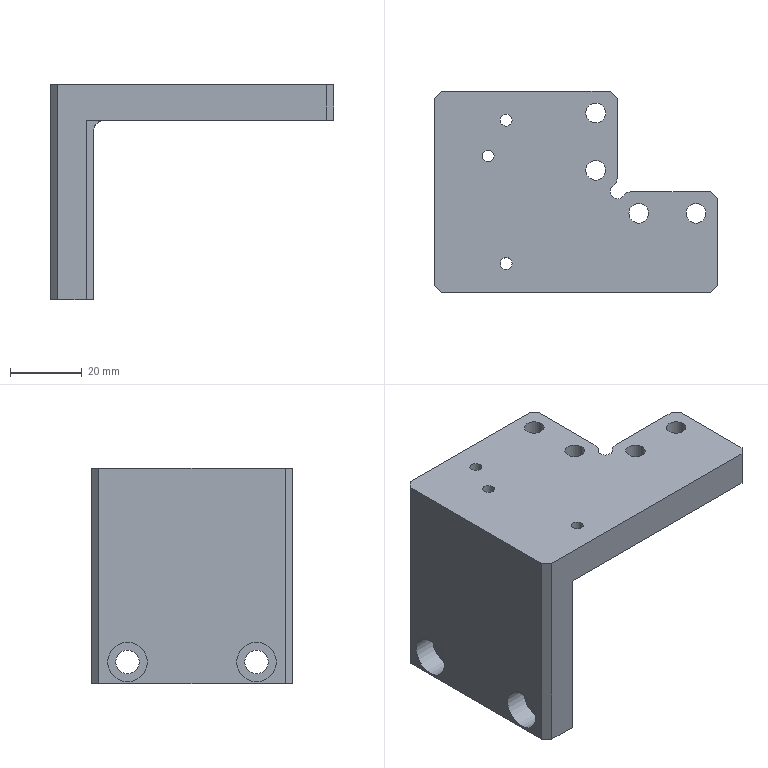Part | 1 solid | 42 faces | box 79 x 56 x 60 mm | volume 65502 mm3 | plane 23 | cylinder 19 | commonest cylinder face diameters 5.5 x4 10 x4 3.3 x3 6 x3 6.6 x2 11 x2
STEP:
#1=CARTESIAN_POINT('',(10.3,1.6,20.));
#2=VERTEX_POINT('',#1);
#3=CARTESIAN_POINT('',(13.1,-1.2,20.));
#4=VERTEX_POINT('',#3);
#5=CARTESIAN_POINT('',(11.5,0.,20.));
#6=DIRECTION('',(0.,0.,1.));
#7=DIRECTION('',(1.,0.,0.));
#8=AXIS2_PLACEMENT_3D('',#5,#6,#7);
#9=CIRCLE('',#8,2.);
#10=EDGE_CURVE('',#2,#4,#9,.T.);
#11=ORIENTED_EDGE('',*,*,#10,.F.);
#12=CARTESIAN_POINT('',(10.3,1.6,30.));
#13=VERTEX_POINT('',#12);
#14=CARTESIAN_POINT('',(10.3,1.6,20.));
#15=DIRECTION('',(0.,0.,1.));
#16=VECTOR('',#15,1000.);
#17=LINE('',#14,#16);
#18=EDGE_CURVE('',#2,#13,#17,.T.);
#19=ORIENTED_EDGE('',*,*,#18,.T.);
#20=CARTESIAN_POINT('',(13.1,-1.2,30.));
#21=VERTEX_POINT('',#20);
#22=CARTESIAN_POINT('',(11.5,0.,30.));
#23=DIRECTION('',(0.,0.,1.));
#24=DIRECTION('',(1.,0.,0.));
#25=AXIS2_PLACEMENT_3D('',#22,#23,#24);
#26=CIRCLE('',#25,2.);
#27=EDGE_CURVE('',#13,#21,#26,.T.);
#28=ORIENTED_EDGE('',*,*,#27,.T.);
#29=CARTESIAN_POINT('',(13.1,-1.2,20.));
#30=DIRECTION('',(0.,0.,1.));
#31=VECTOR('',#30,1000.);
#32=LINE('',#29,#31);
#33=EDGE_CURVE('',#21,#4,#32,.F.);
#34=ORIENTED_EDGE('',*,*,#33,.T.);
#35=EDGE_LOOP('',(#11,#19,#28,#34));
#36=FACE_BOUND('',#35,.T.);
#37=CARTESIAN_POINT('',(11.5,0.,20.));
#38=DIRECTION('',(0.,0.,1.));
#39=DIRECTION('',(1.,0.,0.));
#40=AXIS2_PLACEMENT_3D('',#37,#38,#39);
#41=CYLINDRICAL_SURFACE('',#40,2.);
#42=ADVANCED_FACE('',(#36),#41,.F.);
#43=CARTESIAN_POINT('',(-33.1,18.,-29.5));
#44=VERTEX_POINT('',#43);
#45=CARTESIAN_POINT('',(-33.1,18.,-24.));
#46=DIRECTION('',(-1.,0.,0.));
#47=DIRECTION('',(0.,0.,-1.));
#48=AXIS2_PLACEMENT_3D('',#45,#46,#47);
#49=CIRCLE('',#48,5.5);
#50=EDGE_CURVE('',#44,#44,#49,.T.);
#51=ORIENTED_EDGE('',*,*,#50,.T.);
#52=EDGE_LOOP('',(#51));
#53=FACE_BOUND('',#52,.T.);
#54=CARTESIAN_POINT('',(-33.1,18.,-27.3));
#55=VERTEX_POINT('',#54);
#56=CARTESIAN_POINT('',(-33.1,18.,-24.));
#57=DIRECTION('',(-1.,0.,0.));
#58=DIRECTION('',(0.,0.,-1.));
#59=AXIS2_PLACEMENT_3D('',#56,#57,#58);
#60=CIRCLE('',#59,3.3);
#61=EDGE_CURVE('',#55,#55,#60,.T.);
#62=ORIENTED_EDGE('',*,*,#61,.F.);
#63=EDGE_LOOP('',(#62));
#64=FACE_BOUND('',#63,.T.);
#65=CARTESIAN_POINT('',(-33.1,-14.7,-24.));
#66=DIRECTION('',(1.,0.,0.));
#67=DIRECTION('',(0.,0.,-1.));
#68=AXIS2_PLACEMENT_3D('',#65,#66,#67);
#69=PLANE('',#68);
#70=ADVANCED_FACE('',(#53,#64),#69,.F.);
#71=CARTESIAN_POINT('',(-33.1,-18.,-18.5));
#72=VERTEX_POINT('',#71);
#73=CARTESIAN_POINT('',(-33.1,-18.,-24.));
#74=DIRECTION('',(-1.,0.,0.));
#75=DIRECTION('',(0.,0.,1.));
#76=AXIS2_PLACEMENT_3D('',#73,#74,#75);
#77=CIRCLE('',#76,5.5);
#78=EDGE_CURVE('',#72,#72,#77,.T.);
#79=ORIENTED_EDGE('',*,*,#78,.T.);
#80=EDGE_LOOP('',(#79));
#81=FACE_BOUND('',#80,.T.);
#82=CARTESIAN_POINT('',(-33.1,-18.,-20.7));
#83=VERTEX_POINT('',#82);
#84=CARTESIAN_POINT('',(-33.1,-18.,-24.));
#85=DIRECTION('',(-1.,0.,0.));
#86=DIRECTION('',(0.,0.,1.));
#87=AXIS2_PLACEMENT_3D('',#84,#85,#86);
#88=CIRCLE('',#87,3.3);
#89=EDGE_CURVE('',#83,#83,#88,.T.);
#90=ORIENTED_EDGE('',*,*,#89,.F.);
#91=EDGE_LOOP('',(#90));
#92=FACE_BOUND('',#91,.T.);
#93=CARTESIAN_POINT('',(-33.1,-14.7,-24.));
#94=DIRECTION('',(1.,0.,0.));
#95=DIRECTION('',(0.,0.,-1.));
#96=AXIS2_PLACEMENT_3D('',#93,#94,#95);
#97=PLANE('',#96);
#98=ADVANCED_FACE('',(#81,#92),#97,.F.);
#99=CARTESIAN_POINT('',(-24.5,11.65,20.));
#100=VERTEX_POINT('',#99);
#101=CARTESIAN_POINT('',(-24.5,23.,20.));
#102=VERTEX_POINT('',#101);
#103=CARTESIAN_POINT('',(-24.5,26.,20.));
#104=DIRECTION('',(0.,1.,0.));
#105=VECTOR('',#104,1000.);
#106=LINE('',#103,#105);
#107=EDGE_CURVE('',#100,#102,#106,.T.);
#108=ORIENTED_EDGE('',*,*,#107,.F.);
#109=CARTESIAN_POINT('',(-24.5,8.35,20.));
#110=VERTEX_POINT('',#109);
#111=CARTESIAN_POINT('',(-24.5,11.65,20.));
#112=CARTESIAN_POINT('',(-24.946,11.65,20.));
#113=CARTESIAN_POINT('',(-25.788,11.29,19.774));
#114=CARTESIAN_POINT('',(-26.331,10.001,19.371));
#115=CARTESIAN_POINT('',(-25.788,8.709,19.774));
#116=CARTESIAN_POINT('',(-24.946,8.35,20.));
#117=CARTESIAN_POINT('',(-24.5,8.35,20.));
#118=B_SPLINE_CURVE_WITH_KNOTS('',3,(#111,#112,#113,#114,#115,#116,#117),.UNSPECIFIED.,.F.,.F.,(4,1,1,1,4),(-0.002635,-0.001318,-0.000000456,0.001317,0.002634),.UNSPECIFIED.);
#119=EDGE_CURVE('',#100,#110,#118,.T.);
#120=ORIENTED_EDGE('',*,*,#119,.T.);
#121=CARTESIAN_POINT('',(-24.5,-23.,20.));
#122=VERTEX_POINT('',#121);
#123=CARTESIAN_POINT('',(-24.5,26.,20.));
#124=DIRECTION('',(0.,1.,0.));
#125=VECTOR('',#124,1000.);
#126=LINE('',#123,#125);
#127=EDGE_CURVE('',#122,#110,#126,.T.);
#128=ORIENTED_EDGE('',*,*,#127,.F.);
#129=CARTESIAN_POINT('',(-27.5,-26.,17.));
#130=VERTEX_POINT('',#129);
#131=CARTESIAN_POINT('',(-24.5,-23.,17.));
#132=DIRECTION('',(-0.7071,0.7071,0.));
#133=DIRECTION('',(0.7071,0.7071,0.));
#134=AXIS2_PLACEMENT_3D('',#131,#132,#133);
#135=ELLIPSE('',#134,4.243,3.);
#136=EDGE_CURVE('',#130,#122,#135,.T.);
#137=ORIENTED_EDGE('',*,*,#136,.F.);
#138=CARTESIAN_POINT('',(-27.5,26.,17.));
#139=VERTEX_POINT('',#138);
#140=CARTESIAN_POINT('',(-27.5,-26.,17.));
#141=DIRECTION('',(0.,-1.,0.));
#142=VECTOR('',#141,1000.);
#143=LINE('',#140,#142);
#144=EDGE_CURVE('',#139,#130,#143,.T.);
#145=ORIENTED_EDGE('',*,*,#144,.F.);
#146=CARTESIAN_POINT('',(-24.5,23.,17.));
#147=DIRECTION('',(-0.7071,-0.7071,0.));
#148=DIRECTION('',(-0.7071,0.7071,0.));
#149=AXIS2_PLACEMENT_3D('',#146,#147,#148);
#150=ELLIPSE('',#149,4.243,3.);
#151=EDGE_CURVE('',#102,#139,#150,.T.);
#152=ORIENTED_EDGE('',*,*,#151,.F.);
#153=EDGE_LOOP('',(#108,#120,#128,#137,#145,#152));
#154=FACE_BOUND('',#153,.T.);
#155=CARTESIAN_POINT('',(-24.5,28.,17.));
#156=DIRECTION('',(0.,1.,0.));
#157=DIRECTION('',(0.,0.,1.));
#158=AXIS2_PLACEMENT_3D('',#155,#156,#157);
#159=CYLINDRICAL_SURFACE('',#158,3.);
#160=ADVANCED_FACE('',(#154),#159,.F.);
#161=CARTESIAN_POINT('',(-37.5,28.,30.));
#162=VERTEX_POINT('',#161);
#163=CARTESIAN_POINT('',(-39.5,26.,30.));
#164=VERTEX_POINT('',#163);
#165=CARTESIAN_POINT('',(-32.75,32.75,30.));
#166=DIRECTION('',(-0.7071,-0.7071,0.));
#167=VECTOR('',#166,1000.);
#168=LINE('',#165,#167);
#169=EDGE_CURVE('',#162,#164,#168,.T.);
#170=ORIENTED_EDGE('',*,*,#169,.F.);
#171=CARTESIAN_POINT('',(-37.5,28.,-30.));
#172=VERTEX_POINT('',#171);
#173=CARTESIAN_POINT('',(-37.5,28.,30.));
#174=DIRECTION('',(0.,0.,1.));
#175=VECTOR('',#174,1000.);
#176=LINE('',#173,#175);
#177=EDGE_CURVE('',#172,#162,#176,.T.);
#178=ORIENTED_EDGE('',*,*,#177,.F.);
#179=CARTESIAN_POINT('',(-39.5,26.,-30.));
#180=VERTEX_POINT('',#179);
#181=CARTESIAN_POINT('',(-39.5,26.,-30.));
#182=DIRECTION('',(0.7071,0.7071,0.));
#183=VECTOR('',#182,1000.);
#184=LINE('',#181,#183);
#185=EDGE_CURVE('',#180,#172,#184,.T.);
#186=ORIENTED_EDGE('',*,*,#185,.F.);
#187=CARTESIAN_POINT('',(-39.5,26.,30.));
#188=DIRECTION('',(0.,0.,-1.));
#189=VECTOR('',#188,1000.);
#190=LINE('',#187,#189);
#191=EDGE_CURVE('',#164,#180,#190,.T.);
#192=ORIENTED_EDGE('',*,*,#191,.F.);
#193=EDGE_LOOP('',(#170,#178,#186,#192));
#194=FACE_BOUND('',#193,.T.);
#195=CARTESIAN_POINT('',(-39.5,26.,30.));
#196=DIRECTION('',(0.7071,-0.7071,0.));
#197=DIRECTION('',(0.,0.,-1.));
#198=AXIS2_PLACEMENT_3D('',#195,#196,#197);
#199=PLANE('',#198);
#200=ADVANCED_FACE('',(#194),#199,.F.);
#201=CARTESIAN_POINT('',(-29.5,28.,20.));
#202=VERTEX_POINT('',#201);
#203=CARTESIAN_POINT('',(5.,-6.5,20.));
#204=DIRECTION('',(-0.7071,0.7071,0.));
#205=VECTOR('',#204,1000.);
#206=LINE('',#203,#205);
#207=EDGE_CURVE('',#102,#202,#206,.T.);
#208=ORIENTED_EDGE('',*,*,#207,.F.);
#209=ORIENTED_EDGE('',*,*,#151,.T.);
#210=CARTESIAN_POINT('',(-27.5,26.,-30.));
#211=VERTEX_POINT('',#210);
#212=CARTESIAN_POINT('',(-27.5,26.,-30.));
#213=DIRECTION('',(0.,0.,1.));
#214=VECTOR('',#213,1000.);
#215=LINE('',#212,#214);
#216=EDGE_CURVE('',#211,#139,#215,.T.);
#217=ORIENTED_EDGE('',*,*,#216,.F.);
#218=CARTESIAN_POINT('',(-29.5,28.,-30.));
#219=VERTEX_POINT('',#218);
#220=CARTESIAN_POINT('',(-29.5,28.,-30.));
#221=DIRECTION('',(0.7071,-0.7071,0.));
#222=VECTOR('',#221,1000.);
#223=LINE('',#220,#222);
#224=EDGE_CURVE('',#219,#211,#223,.T.);
#225=ORIENTED_EDGE('',*,*,#224,.F.);
#226=CARTESIAN_POINT('',(-29.5,28.,30.));
#227=DIRECTION('',(0.,0.,-1.));
#228=VECTOR('',#227,1000.);
#229=LINE('',#226,#228);
#230=EDGE_CURVE('',#202,#219,#229,.T.);
#231=ORIENTED_EDGE('',*,*,#230,.F.);
#232=EDGE_LOOP('',(#208,#209,#217,#225,#231));
#233=FACE_BOUND('',#232,.T.);
#234=CARTESIAN_POINT('',(-29.5,28.,30.));
#235=DIRECTION('',(-0.7071,-0.7071,0.));
#236=DIRECTION('',(0.,0.,-1.));
#237=AXIS2_PLACEMENT_3D('',#234,#235,#236);
#238=PLANE('',#237);
#239=ADVANCED_FACE('',(#233),#238,.F.);
#240=CARTESIAN_POINT('',(-39.5,-26.,30.));
#241=VERTEX_POINT('',#240);
#242=CARTESIAN_POINT('',(-37.5,-28.,30.));
#243=VERTEX_POINT('',#242);
#244=CARTESIAN_POINT('',(-32.75,-32.75,30.));
#245=DIRECTION('',(0.7071,-0.7071,0.));
#246=VECTOR('',#245,1000.);
#247=LINE('',#244,#246);
#248=EDGE_CURVE('',#241,#243,#247,.T.);
#249=ORIENTED_EDGE('',*,*,#248,.F.);
#250=CARTESIAN_POINT('',(-39.5,-26.,-30.));
#251=VERTEX_POINT('',#250);
#252=CARTESIAN_POINT('',(-39.5,-26.,30.));
#253=DIRECTION('',(0.,0.,1.));
#254=VECTOR('',#253,1000.);
#255=LINE('',#252,#254);
#256=EDGE_CURVE('',#251,#241,#255,.T.);
#257=ORIENTED_EDGE('',*,*,#256,.F.);
#258=CARTESIAN_POINT('',(-37.5,-28.,-30.));
#259=VERTEX_POINT('',#258);
#260=CARTESIAN_POINT('',(-37.5,-28.,-30.));
#261=DIRECTION('',(-0.7071,0.7071,0.));
#262=VECTOR('',#261,1000.);
#263=LINE('',#260,#262);
#264=EDGE_CURVE('',#259,#251,#263,.T.);
#265=ORIENTED_EDGE('',*,*,#264,.F.);
#266=CARTESIAN_POINT('',(-37.5,-28.,30.));
#267=DIRECTION('',(0.,0.,-1.));
#268=VECTOR('',#267,1000.);
#269=LINE('',#266,#268);
#270=EDGE_CURVE('',#243,#259,#269,.T.);
#271=ORIENTED_EDGE('',*,*,#270,.F.);
#272=EDGE_LOOP('',(#249,#257,#265,#271));
#273=FACE_BOUND('',#272,.T.);
#274=CARTESIAN_POINT('',(-37.5,-28.,30.));
#275=DIRECTION('',(0.7071,0.7071,0.));
#276=DIRECTION('',(0.,0.,-1.));
#277=AXIS2_PLACEMENT_3D('',#274,#275,#276);
#278=PLANE('',#277);
#279=ADVANCED_FACE('',(#273),#278,.F.);
#280=CARTESIAN_POINT('',(-29.5,-28.,20.));
#281=VERTEX_POINT('',#280);
#282=CARTESIAN_POINT('',(33.,34.5,20.));
#283=DIRECTION('',(0.7071,0.7071,0.));
#284=VECTOR('',#283,1000.);
#285=LINE('',#282,#284);
#286=EDGE_CURVE('',#281,#122,#285,.T.);
#287=ORIENTED_EDGE('',*,*,#286,.F.);
#288=CARTESIAN_POINT('',(-29.5,-28.,-30.));
#289=VERTEX_POINT('',#288);
#290=CARTESIAN_POINT('',(-29.5,-28.,30.));
#291=DIRECTION('',(0.,0.,1.));
#292=VECTOR('',#291,1000.);
#293=LINE('',#290,#292);
#294=EDGE_CURVE('',#289,#281,#293,.T.);
#295=ORIENTED_EDGE('',*,*,#294,.F.);
#296=CARTESIAN_POINT('',(-27.5,-26.,-30.));
#297=VERTEX_POINT('',#296);
#298=CARTESIAN_POINT('',(-27.5,-26.,-30.));
#299=DIRECTION('',(-0.7071,-0.7071,0.));
#300=VECTOR('',#299,1000.);
#301=LINE('',#298,#300);
#302=EDGE_CURVE('',#297,#289,#301,.T.);
#303=ORIENTED_EDGE('',*,*,#302,.F.);
#304=CARTESIAN_POINT('',(-27.5,-26.,-30.));
#305=DIRECTION('',(0.,0.,-1.));
#306=VECTOR('',#305,1000.);
#307=LINE('',#304,#306);
#308=EDGE_CURVE('',#130,#297,#307,.T.);
#309=ORIENTED_EDGE('',*,*,#308,.F.);
#310=ORIENTED_EDGE('',*,*,#136,.T.);
#311=EDGE_LOOP('',(#287,#295,#303,#309,#310));
#312=FACE_BOUND('',#311,.T.);
#313=CARTESIAN_POINT('',(-27.5,-26.,-30.));
#314=DIRECTION('',(-0.7071,0.7071,0.));
#315=DIRECTION('',(0.,0.,-1.));
#316=AXIS2_PLACEMENT_3D('',#313,#314,#315);
#317=PLANE('',#316);
#318=ADVANCED_FACE('',(#312),#317,.F.);
#319=CARTESIAN_POINT('',(37.5,-28.,30.));
#320=VERTEX_POINT('',#319);
#321=CARTESIAN_POINT('',(39.5,-26.,30.));
#322=VERTEX_POINT('',#321);
#323=CARTESIAN_POINT('',(32.75,-32.75,30.));
#324=DIRECTION('',(0.7071,0.7071,0.));
#325=VECTOR('',#324,1000.);
#326=LINE('',#323,#325);
#327=EDGE_CURVE('',#320,#322,#326,.T.);
#328=ORIENTED_EDGE('',*,*,#327,.F.);
#329=CARTESIAN_POINT('',(37.5,-28.,20.));
#330=VERTEX_POINT('',#329);
#331=CARTESIAN_POINT('',(37.5,-28.,30.));
#332=DIRECTION('',(0.,0.,1.));
#333=VECTOR('',#332,1000.);
#334=LINE('',#331,#333);
#335=EDGE_CURVE('',#330,#320,#334,.T.);
#336=ORIENTED_EDGE('',*,*,#335,.F.);
#337=CARTESIAN_POINT('',(39.5,-26.,20.));
#338=VERTEX_POINT('',#337);
#339=CARTESIAN_POINT('',(39.5,-26.,20.));
#340=DIRECTION('',(-0.7071,-0.7071,0.));
#341=VECTOR('',#340,1000.);
#342=LINE('',#339,#341);
#343=EDGE_CURVE('',#338,#330,#342,.T.);
#344=ORIENTED_EDGE('',*,*,#343,.F.);
#345=CARTESIAN_POINT('',(39.5,-26.,30.));
#346=DIRECTION('',(0.,0.,-1.));
#347=VECTOR('',#346,1000.);
#348=LINE('',#345,#347);
#349=EDGE_CURVE('',#322,#338,#348,.T.);
#350=ORIENTED_EDGE('',*,*,#349,.F.);
#351=EDGE_LOOP('',(#328,#336,#344,#350));
#352=FACE_BOUND('',#351,.T.);
#353=CARTESIAN_POINT('',(39.5,-26.,30.));
#354=DIRECTION('',(-0.7071,0.7071,0.));
#355=DIRECTION('',(0.,0.,-1.));
#356=AXIS2_PLACEMENT_3D('',#353,#354,#355);
#357=PLANE('',#356);
#358=ADVANCED_FACE('',(#352),#357,.F.);
#359=CARTESIAN_POINT('',(37.5,0.,20.));
#360=VERTEX_POINT('',#359);
#361=CARTESIAN_POINT('',(39.5,-2.,20.));
#362=VERTEX_POINT('',#361);
#363=CARTESIAN_POINT('',(24.5,13.,20.));
#364=DIRECTION('',(0.7071,-0.7071,0.));
#365=VECTOR('',#364,1000.);
#366=LINE('',#363,#365);
#367=EDGE_CURVE('',#360,#362,#366,.T.);
#368=ORIENTED_EDGE('',*,*,#367,.F.);
#369=CARTESIAN_POINT('',(37.5,0.,30.));
#370=VERTEX_POINT('',#369);
#371=CARTESIAN_POINT('',(37.5,0.,-30.));
#372=DIRECTION('',(0.,0.,-1.));
#373=VECTOR('',#372,1000.);
#374=LINE('',#371,#373);
#375=EDGE_CURVE('',#370,#360,#374,.T.);
#376=ORIENTED_EDGE('',*,*,#375,.F.);
#377=CARTESIAN_POINT('',(39.5,-2.,30.));
#378=VERTEX_POINT('',#377);
#379=CARTESIAN_POINT('',(18.75,18.75,30.));
#380=DIRECTION('',(-0.7071,0.7071,0.));
#381=VECTOR('',#380,1000.);
#382=LINE('',#379,#381);
#383=EDGE_CURVE('',#378,#370,#382,.T.);
#384=ORIENTED_EDGE('',*,*,#383,.F.);
#385=CARTESIAN_POINT('',(39.5,-2.,30.));
#386=DIRECTION('',(0.,0.,1.));
#387=VECTOR('',#386,1000.);
#388=LINE('',#385,#387);
#389=EDGE_CURVE('',#362,#378,#388,.T.);
#390=ORIENTED_EDGE('',*,*,#389,.F.);
#391=EDGE_LOOP('',(#368,#376,#384,#390));
#392=FACE_BOUND('',#391,.T.);
#393=CARTESIAN_POINT('',(11.5,26.,-30.));
#394=DIRECTION('',(-0.7071,-0.7071,0.));
#395=DIRECTION('',(0.,0.,1.));
#396=AXIS2_PLACEMENT_3D('',#393,#394,#395);
#397=PLANE('',#396);
#398=ADVANCED_FACE('',(#392),#397,.F.);
#399=CARTESIAN_POINT('',(9.5,28.,20.));
#400=VERTEX_POINT('',#399);
#401=CARTESIAN_POINT('',(11.5,26.,20.));
#402=VERTEX_POINT('',#401);
#403=CARTESIAN_POINT('',(11.5,26.,20.));
#404=DIRECTION('',(0.7071,-0.7071,0.));
#405=VECTOR('',#404,1000.);
#406=LINE('',#403,#405);
#407=EDGE_CURVE('',#400,#402,#406,.T.);
#408=ORIENTED_EDGE('',*,*,#407,.F.);
#409=CARTESIAN_POINT('',(9.5,28.,30.));
#410=VERTEX_POINT('',#409);
#411=CARTESIAN_POINT('',(9.5,28.,30.));
#412=DIRECTION('',(0.,0.,-1.));
#413=VECTOR('',#412,1000.);
#414=LINE('',#411,#413);
#415=EDGE_CURVE('',#410,#400,#414,.T.);
#416=ORIENTED_EDGE('',*,*,#415,.F.);
#417=CARTESIAN_POINT('',(11.5,26.,30.));
#418=VERTEX_POINT('',#417);
#419=CARTESIAN_POINT('',(18.75,18.75,30.));
#420=DIRECTION('',(-0.7071,0.7071,0.));
#421=VECTOR('',#420,1000.);
#422=LINE('',#419,#421);
#423=EDGE_CURVE('',#418,#410,#422,.T.);
#424=ORIENTED_EDGE('',*,*,#423,.F.);
#425=CARTESIAN_POINT('',(11.5,26.,-30.));
#426=DIRECTION('',(0.,0.,1.));
#427=VECTOR('',#426,1000.);
#428=LINE('',#425,#427);
#429=EDGE_CURVE('',#402,#418,#428,.T.);
#430=ORIENTED_EDGE('',*,*,#429,.F.);
#431=EDGE_LOOP('',(#408,#416,#424,#430));
#432=FACE_BOUND('',#431,.T.);
#433=CARTESIAN_POINT('',(11.5,26.,-30.));
#434=DIRECTION('',(-0.7071,-0.7071,0.));
#435=DIRECTION('',(0.,0.,1.));
#436=AXIS2_PLACEMENT_3D('',#433,#434,#435);
#437=PLANE('',#436);
#438=ADVANCED_FACE('',(#432),#437,.F.);
#439=CARTESIAN_POINT('',(10.5,22.,25.4));
#440=VERTEX_POINT('',#439);
#441=CARTESIAN_POINT('',(5.5,22.,25.4));
#442=DIRECTION('',(0.,0.,-1.));
#443=DIRECTION('',(1.,0.,0.));
#444=AXIS2_PLACEMENT_3D('',#441,#442,#443);
#445=CIRCLE('',#444,5.);
#446=EDGE_CURVE('',#440,#440,#445,.T.);
#447=ORIENTED_EDGE('',*,*,#446,.T.);
#448=EDGE_LOOP('',(#447));
#449=FACE_BOUND('',#448,.T.);
#450=CARTESIAN_POINT('',(8.25,22.,25.4));
#451=VERTEX_POINT('',#450);
#452=CARTESIAN_POINT('',(5.5,22.,25.4));
#453=DIRECTION('',(0.,0.,-1.));
#454=DIRECTION('',(1.,0.,0.));
#455=AXIS2_PLACEMENT_3D('',#452,#453,#454);
#456=CIRCLE('',#455,2.75);
#457=EDGE_CURVE('',#451,#451,#456,.T.);
#458=ORIENTED_EDGE('',*,*,#457,.F.);
#459=EDGE_LOOP('',(#458));
#460=FACE_BOUND('',#459,.T.);
#461=CARTESIAN_POINT('',(36.25,-6.,25.4));
#462=DIRECTION('',(0.,0.,1.));
#463=DIRECTION('',(1.,0.,0.));
#464=AXIS2_PLACEMENT_3D('',#461,#462,#463);
#465=PLANE('',#464);
#466=ADVANCED_FACE('',(#449,#460),#465,.F.);
#467=CARTESIAN_POINT('',(10.5,6.,25.4));
#468=VERTEX_POINT('',#467);
#469=CARTESIAN_POINT('',(5.5,6.,25.4));
#470=DIRECTION('',(0.,0.,-1.));
#471=DIRECTION('',(1.,0.,0.));
#472=AXIS2_PLACEMENT_3D('',#469,#470,#471);
#473=CIRCLE('',#472,5.);
#474=EDGE_CURVE('',#468,#468,#473,.T.);
#475=ORIENTED_EDGE('',*,*,#474,.T.);
#476=EDGE_LOOP('',(#475));
#477=FACE_BOUND('',#476,.T.);
#478=CARTESIAN_POINT('',(8.25,6.,25.4));
#479=VERTEX_POINT('',#478);
#480=CARTESIAN_POINT('',(5.5,6.,25.4));
#481=DIRECTION('',(0.,0.,-1.));
#482=DIRECTION('',(1.,0.,0.));
#483=AXIS2_PLACEMENT_3D('',#480,#481,#482);
#484=CIRCLE('',#483,2.75);
#485=EDGE_CURVE('',#479,#479,#484,.T.);
#486=ORIENTED_EDGE('',*,*,#485,.F.);
#487=EDGE_LOOP('',(#486));
#488=FACE_BOUND('',#487,.T.);
#489=CARTESIAN_POINT('',(36.25,-6.,25.4));
#490=DIRECTION('',(0.,0.,1.));
#491=DIRECTION('',(1.,0.,0.));
#492=AXIS2_PLACEMENT_3D('',#489,#490,#491);
#493=PLANE('',#492);
#494=ADVANCED_FACE('',(#477,#488),#493,.F.);
#495=CARTESIAN_POINT('',(22.5,-6.,25.4));
#496=VERTEX_POINT('',#495);
#497=CARTESIAN_POINT('',(17.5,-6.,25.4));
#498=DIRECTION('',(0.,0.,-1.));
#499=DIRECTION('',(1.,0.,0.));
#500=AXIS2_PLACEMENT_3D('',#497,#498,#499);
#501=CIRCLE('',#500,5.);
#502=EDGE_CURVE('',#496,#496,#501,.T.);
#503=ORIENTED_EDGE('',*,*,#502,.T.);
#504=EDGE_LOOP('',(#503));
#505=FACE_BOUND('',#504,.T.);
#506=CARTESIAN_POINT('',(20.25,-6.,25.4));
#507=VERTEX_POINT('',#506);
#508=CARTESIAN_POINT('',(17.5,-6.,25.4));
#509=DIRECTION('',(0.,0.,-1.));
#510=DIRECTION('',(1.,0.,0.));
#511=AXIS2_PLACEMENT_3D('',#508,#509,#510);
#512=CIRCLE('',#511,2.75);
#513=EDGE_CURVE('',#507,#507,#512,.T.);
#514=ORIENTED_EDGE('',*,*,#513,.F.);
#515=EDGE_LOOP('',(#514));
#516=FACE_BOUND('',#515,.T.);
#517=CARTESIAN_POINT('',(36.25,-6.,25.4));
#518=DIRECTION('',(0.,0.,1.));
#519=DIRECTION('',(1.,0.,0.));
#520=AXIS2_PLACEMENT_3D('',#517,#518,#519);
#521=PLANE('',#520);
#522=ADVANCED_FACE('',(#505,#516),#521,.F.);
#523=CARTESIAN_POINT('',(28.5,-6.,25.4));
#524=VERTEX_POINT('',#523);
#525=CARTESIAN_POINT('',(33.5,-6.,25.4));
#526=DIRECTION('',(0.,0.,-1.));
#527=DIRECTION('',(-1.,0.,0.));
#528=AXIS2_PLACEMENT_3D('',#525,#526,#527);
#529=CIRCLE('',#528,5.);
#530=EDGE_CURVE('',#524,#524,#529,.T.);
#531=ORIENTED_EDGE('',*,*,#530,.T.);
#532=EDGE_LOOP('',(#531));
#533=FACE_BOUND('',#532,.T.);
#534=CARTESIAN_POINT('',(30.75,-6.,25.4));
#535=VERTEX_POINT('',#534);
#536=CARTESIAN_POINT('',(33.5,-6.,25.4));
#537=DIRECTION('',(0.,0.,-1.));
#538=DIRECTION('',(-1.,0.,0.));
#539=AXIS2_PLACEMENT_3D('',#536,#537,#538);
#540=CIRCLE('',#539,2.75);
#541=EDGE_CURVE('',#535,#535,#540,.T.);
#542=ORIENTED_EDGE('',*,*,#541,.F.);
#543=EDGE_LOOP('',(#542));
#544=FACE_BOUND('',#543,.T.);
#545=CARTESIAN_POINT('',(36.25,-6.,25.4));
#546=DIRECTION('',(0.,0.,1.));
#547=DIRECTION('',(1.,0.,0.));
#548=AXIS2_PLACEMENT_3D('',#545,#546,#547);
#549=PLANE('',#548);
#550=ADVANCED_FACE('',(#533,#544),#549,.F.);
#551=CARTESIAN_POINT('',(11.5,4.,30.));
#552=VERTEX_POINT('',#551);
#553=CARTESIAN_POINT('',(11.5,0.,30.));
#554=DIRECTION('',(0.,-1.,0.));
#555=VECTOR('',#554,1000.);
#556=LINE('',#553,#555);
#557=EDGE_CURVE('',#418,#552,#556,.T.);
#558=ORIENTED_EDGE('',*,*,#557,.T.);
#559=CARTESIAN_POINT('',(11.5,4.,20.));
#560=VERTEX_POINT('',#559);
#561=CARTESIAN_POINT('',(11.5,4.,-30.));
#562=DIRECTION('',(0.,0.,1.));
#563=VECTOR('',#562,1000.);
#564=LINE('',#561,#563);
#565=EDGE_CURVE('',#552,#560,#564,.F.);
#566=ORIENTED_EDGE('',*,*,#565,.T.);
#567=CARTESIAN_POINT('',(11.5,28.,20.));
#568=DIRECTION('',(0.,-1.,0.));
#569=VECTOR('',#568,1000.);
#570=LINE('',#567,#569);
#571=EDGE_CURVE('',#402,#560,#570,.T.);
#572=ORIENTED_EDGE('',*,*,#571,.F.);
#573=ORIENTED_EDGE('',*,*,#429,.T.);
#574=EDGE_LOOP('',(#558,#566,#572,#573));
#575=FACE_BOUND('',#574,.T.);
#576=CARTESIAN_POINT('',(11.5,0.,-30.));
#577=DIRECTION('',(-1.,0.,0.));
#578=DIRECTION('',(0.,0.,1.));
#579=AXIS2_PLACEMENT_3D('',#576,#577,#578);
#580=PLANE('',#579);
#581=ADVANCED_FACE('',(#575),#580,.F.);
#582=CARTESIAN_POINT('',(15.5,0.,20.));
#583=VERTEX_POINT('',#582);
#584=CARTESIAN_POINT('',(39.5,0.,20.));
#585=DIRECTION('',(1.,0.,0.));
#586=VECTOR('',#585,1000.);
#587=LINE('',#584,#586);
#588=EDGE_CURVE('',#583,#360,#587,.T.);
#589=ORIENTED_EDGE('',*,*,#588,.F.);
#590=CARTESIAN_POINT('',(15.5,0.,30.));
#591=VERTEX_POINT('',#590);
#592=CARTESIAN_POINT('',(15.5,0.,-30.));
#593=DIRECTION('',(0.,0.,1.));
#594=VECTOR('',#593,1000.);
#595=LINE('',#592,#594);
#596=EDGE_CURVE('',#583,#591,#595,.T.);
#597=ORIENTED_EDGE('',*,*,#596,.T.);
#598=CARTESIAN_POINT('',(39.5,0.,30.));
#599=DIRECTION('',(1.,0.,0.));
#600=VECTOR('',#599,1000.);
#601=LINE('',#598,#600);
#602=EDGE_CURVE('',#591,#370,#601,.T.);
#603=ORIENTED_EDGE('',*,*,#602,.T.);
#604=ORIENTED_EDGE('',*,*,#375,.T.);
#605=EDGE_LOOP('',(#589,#597,#603,#604));
#606=FACE_BOUND('',#605,.T.);
#607=CARTESIAN_POINT('',(39.5,0.,-30.));
#608=DIRECTION('',(0.,-1.,0.));
#609=DIRECTION('',(1.,0.,0.));
#610=AXIS2_PLACEMENT_3D('',#607,#608,#609);
#611=PLANE('',#610);
#612=ADVANCED_FACE('',(#606),#611,.F.);
#613=ORIENTED_EDGE('',*,*,#571,.T.);
#614=CARTESIAN_POINT('',(8.5,4.,20.));
#615=DIRECTION('',(0.,0.,1.));
#616=DIRECTION('',(1.,0.,0.));
#617=AXIS2_PLACEMENT_3D('',#614,#615,#616);
#618=CIRCLE('',#617,3.);
#619=EDGE_CURVE('',#560,#2,#618,.F.);
#620=ORIENTED_EDGE('',*,*,#619,.T.);
#621=ORIENTED_EDGE('',*,*,#10,.T.);
#622=CARTESIAN_POINT('',(15.5,-3.,20.));
#623=DIRECTION('',(0.,0.,1.));
#624=DIRECTION('',(1.,0.,0.));
#625=AXIS2_PLACEMENT_3D('',#622,#623,#624);
#626=CIRCLE('',#625,3.);
#627=EDGE_CURVE('',#4,#583,#626,.F.);
#628=ORIENTED_EDGE('',*,*,#627,.T.);
#629=ORIENTED_EDGE('',*,*,#588,.T.);
#630=ORIENTED_EDGE('',*,*,#367,.T.);
#631=CARTESIAN_POINT('',(39.5,28.,20.));
#632=DIRECTION('',(0.,-1.,0.));
#633=VECTOR('',#632,1000.);
#634=LINE('',#631,#633);
#635=EDGE_CURVE('',#362,#338,#634,.T.);
#636=ORIENTED_EDGE('',*,*,#635,.T.);
#637=ORIENTED_EDGE('',*,*,#343,.T.);
#638=CARTESIAN_POINT('',(39.5,-28.,20.));
#639=DIRECTION('',(-1.,0.,0.));
#640=VECTOR('',#639,1000.);
#641=LINE('',#638,#640);
#642=EDGE_CURVE('',#330,#281,#641,.T.);
#643=ORIENTED_EDGE('',*,*,#642,.T.);
#644=ORIENTED_EDGE('',*,*,#286,.T.);
#645=ORIENTED_EDGE('',*,*,#127,.T.);
#646=CARTESIAN_POINT('',(-24.5,10.,20.));
#647=DIRECTION('',(0.,0.,1.));
#648=DIRECTION('',(1.,0.,0.));
#649=AXIS2_PLACEMENT_3D('',#646,#647,#648);
#650=CIRCLE('',#649,1.65);
#651=EDGE_CURVE('',#110,#100,#650,.T.);
#652=ORIENTED_EDGE('',*,*,#651,.T.);
#653=ORIENTED_EDGE('',*,*,#107,.T.);
#654=ORIENTED_EDGE('',*,*,#207,.T.);
#655=CARTESIAN_POINT('',(39.5,28.,20.));
#656=DIRECTION('',(-1.,0.,0.));
#657=VECTOR('',#656,1000.);
#658=LINE('',#655,#657);
#659=EDGE_CURVE('',#400,#202,#658,.T.);
#660=ORIENTED_EDGE('',*,*,#659,.F.);
#661=ORIENTED_EDGE('',*,*,#407,.T.);
#662=EDGE_LOOP('',(#613,#620,#621,#628,#629,#630,#636,#637,#643,#644,#645,#652,#653,#654,#660,#661));
#663=FACE_BOUND('',#662,.T.);
#664=CARTESIAN_POINT('',(28.5,-6.,20.));
#665=VERTEX_POINT('',#664);
#666=CARTESIAN_POINT('',(33.5,-6.,20.));
#667=DIRECTION('',(0.,0.,-1.));
#668=DIRECTION('',(-1.,0.,0.));
#669=AXIS2_PLACEMENT_3D('',#666,#667,#668);
#670=CIRCLE('',#669,5.);
#671=EDGE_CURVE('',#665,#665,#670,.T.);
#672=ORIENTED_EDGE('',*,*,#671,.F.);
#673=EDGE_LOOP('',(#672));
#674=FACE_BOUND('',#673,.T.);
#675=CARTESIAN_POINT('',(12.5,-6.,20.));
#676=VERTEX_POINT('',#675);
#677=CARTESIAN_POINT('',(17.5,-6.,20.));
#678=DIRECTION('',(0.,0.,-1.));
#679=DIRECTION('',(-1.,0.,0.));
#680=AXIS2_PLACEMENT_3D('',#677,#678,#679);
#681=CIRCLE('',#680,5.);
#682=EDGE_CURVE('',#676,#676,#681,.T.);
#683=ORIENTED_EDGE('',*,*,#682,.F.);
#684=EDGE_LOOP('',(#683));
#685=FACE_BOUND('',#684,.T.);
#686=CARTESIAN_POINT('',(0.5,6.,20.));
#687=VERTEX_POINT('',#686);
#688=CARTESIAN_POINT('',(5.5,6.,20.));
#689=DIRECTION('',(0.,0.,-1.));
#690=DIRECTION('',(-1.,0.,0.));
#691=AXIS2_PLACEMENT_3D('',#688,#689,#690);
#692=CIRCLE('',#691,5.);
#693=EDGE_CURVE('',#687,#687,#692,.T.);
#694=ORIENTED_EDGE('',*,*,#693,.F.);
#695=EDGE_LOOP('',(#694));
#696=FACE_BOUND('',#695,.T.);
#697=CARTESIAN_POINT('',(0.5,22.,20.));
#698=VERTEX_POINT('',#697);
#699=CARTESIAN_POINT('',(5.5,22.,20.));
#700=DIRECTION('',(0.,0.,-1.));
#701=DIRECTION('',(-1.,0.,0.));
#702=AXIS2_PLACEMENT_3D('',#699,#700,#701);
#703=CIRCLE('',#702,5.);
#704=EDGE_CURVE('',#698,#698,#703,.T.);
#705=ORIENTED_EDGE('',*,*,#704,.F.);
#706=EDGE_LOOP('',(#705));
#707=FACE_BOUND('',#706,.T.);
#708=CARTESIAN_POINT('',(-17.85,-20.,20.));
#709=VERTEX_POINT('',#708);
#710=CARTESIAN_POINT('',(-19.5,-20.,20.));
#711=DIRECTION('',(0.,0.,1.));
#712=DIRECTION('',(1.,0.,0.));
#713=AXIS2_PLACEMENT_3D('',#710,#711,#712);
#714=CIRCLE('',#713,1.65);
#715=EDGE_CURVE('',#709,#709,#714,.T.);
#716=ORIENTED_EDGE('',*,*,#715,.T.);
#717=EDGE_LOOP('',(#716));
#718=FACE_BOUND('',#717,.T.);
#719=CARTESIAN_POINT('',(-17.85,20.,20.));
#720=VERTEX_POINT('',#719);
#721=CARTESIAN_POINT('',(-19.5,20.,20.));
#722=DIRECTION('',(0.,0.,1.));
#723=DIRECTION('',(1.,0.,0.));
#724=AXIS2_PLACEMENT_3D('',#721,#722,#723);
#725=CIRCLE('',#724,1.65);
#726=EDGE_CURVE('',#720,#720,#725,.T.);
#727=ORIENTED_EDGE('',*,*,#726,.T.);
#728=EDGE_LOOP('',(#727));
#729=FACE_BOUND('',#728,.T.);
#730=CARTESIAN_POINT('',(39.5,28.,20.));
#731=DIRECTION('',(0.,0.,1.));
#732=DIRECTION('',(1.,0.,0.));
#733=AXIS2_PLACEMENT_3D('',#730,#731,#732);
#734=PLANE('',#733);
#735=ADVANCED_FACE('',(#663,#674,#685,#696,#707,#718,#729),#734,.F.);
#736=ORIENTED_EDGE('',*,*,#216,.T.);
#737=ORIENTED_EDGE('',*,*,#144,.T.);
#738=ORIENTED_EDGE('',*,*,#308,.T.);
#739=CARTESIAN_POINT('',(-27.5,28.,-30.));
#740=DIRECTION('',(0.,-1.,0.));
#741=VECTOR('',#740,1000.);
#742=LINE('',#739,#741);
#743=EDGE_CURVE('',#211,#297,#742,.T.);
#744=ORIENTED_EDGE('',*,*,#743,.F.);
#745=EDGE_LOOP('',(#736,#737,#738,#744));
#746=FACE_BOUND('',#745,.T.);
#747=CARTESIAN_POINT('',(-27.5,-18.,-20.7));
#748=VERTEX_POINT('',#747);
#749=CARTESIAN_POINT('',(-27.5,-18.,-24.));
#750=DIRECTION('',(-1.,0.,0.));
#751=DIRECTION('',(0.,0.,1.));
#752=AXIS2_PLACEMENT_3D('',#749,#750,#751);
#753=CIRCLE('',#752,3.3);
#754=EDGE_CURVE('',#748,#748,#753,.T.);
#755=ORIENTED_EDGE('',*,*,#754,.T.);
#756=EDGE_LOOP('',(#755));
#757=FACE_BOUND('',#756,.T.);
#758=CARTESIAN_POINT('',(-27.5,18.,-20.7));
#759=VERTEX_POINT('',#758);
#760=CARTESIAN_POINT('',(-27.5,18.,-24.));
#761=DIRECTION('',(-1.,0.,0.));
#762=DIRECTION('',(0.,0.,1.));
#763=AXIS2_PLACEMENT_3D('',#760,#761,#762);
#764=CIRCLE('',#763,3.3);
#765=EDGE_CURVE('',#759,#759,#764,.T.);
#766=ORIENTED_EDGE('',*,*,#765,.T.);
#767=EDGE_LOOP('',(#766));
#768=FACE_BOUND('',#767,.T.);
#769=CARTESIAN_POINT('',(-27.5,28.,-30.));
#770=DIRECTION('',(-1.,0.,0.));
#771=DIRECTION('',(0.,0.,1.));
#772=AXIS2_PLACEMENT_3D('',#769,#770,#771);
#773=PLANE('',#772);
#774=ADVANCED_FACE('',(#746,#757,#768),#773,.F.);
#775=ORIENTED_EDGE('',*,*,#743,.T.);
#776=ORIENTED_EDGE('',*,*,#302,.T.);
#777=CARTESIAN_POINT('',(-39.5,-28.,-30.));
#778=DIRECTION('',(1.,0.,0.));
#779=VECTOR('',#778,1000.);
#780=LINE('',#777,#779);
#781=EDGE_CURVE('',#259,#289,#780,.T.);
#782=ORIENTED_EDGE('',*,*,#781,.F.);
#783=ORIENTED_EDGE('',*,*,#264,.T.);
#784=CARTESIAN_POINT('',(-39.5,28.,-30.));
#785=DIRECTION('',(0.,-1.,0.));
#786=VECTOR('',#785,1000.);
#787=LINE('',#784,#786);
#788=EDGE_CURVE('',#180,#251,#787,.T.);
#789=ORIENTED_EDGE('',*,*,#788,.F.);
#790=ORIENTED_EDGE('',*,*,#185,.T.);
#791=CARTESIAN_POINT('',(-39.5,28.,-30.));
#792=DIRECTION('',(-1.,0.,0.));
#793=VECTOR('',#792,1000.);
#794=LINE('',#791,#793);
#795=EDGE_CURVE('',#219,#172,#794,.T.);
#796=ORIENTED_EDGE('',*,*,#795,.F.);
#797=ORIENTED_EDGE('',*,*,#224,.T.);
#798=EDGE_LOOP('',(#775,#776,#782,#783,#789,#790,#796,#797));
#799=FACE_BOUND('',#798,.T.);
#800=CARTESIAN_POINT('',(0.,0.,-30.));
#801=DIRECTION('',(0.,0.,1.));
#802=DIRECTION('',(1.,0.,0.));
#803=AXIS2_PLACEMENT_3D('',#800,#801,#802);
#804=PLANE('',#803);
#805=ADVANCED_FACE('',(#799),#804,.F.);
#806=CARTESIAN_POINT('',(36.25,-6.,30.));
#807=VERTEX_POINT('',#806);
#808=CARTESIAN_POINT('',(33.5,-6.,30.));
#809=DIRECTION('',(0.,0.,1.));
#810=DIRECTION('',(1.,0.,0.));
#811=AXIS2_PLACEMENT_3D('',#808,#809,#810);
#812=CIRCLE('',#811,2.75);
#813=EDGE_CURVE('',#807,#807,#812,.T.);
#814=ORIENTED_EDGE('',*,*,#813,.F.);
#815=EDGE_LOOP('',(#814));
#816=FACE_BOUND('',#815,.T.);
#817=CARTESIAN_POINT('',(20.25,-6.,30.));
#818=VERTEX_POINT('',#817);
#819=CARTESIAN_POINT('',(17.5,-6.,30.));
#820=DIRECTION('',(0.,0.,1.));
#821=DIRECTION('',(1.,0.,0.));
#822=AXIS2_PLACEMENT_3D('',#819,#820,#821);
#823=CIRCLE('',#822,2.75);
#824=EDGE_CURVE('',#818,#818,#823,.T.);
#825=ORIENTED_EDGE('',*,*,#824,.F.);
#826=EDGE_LOOP('',(#825));
#827=FACE_BOUND('',#826,.T.);
#828=CARTESIAN_POINT('',(8.25,6.,30.));
#829=VERTEX_POINT('',#828);
#830=CARTESIAN_POINT('',(5.5,6.,30.));
#831=DIRECTION('',(0.,0.,1.));
#832=DIRECTION('',(1.,0.,0.));
#833=AXIS2_PLACEMENT_3D('',#830,#831,#832);
#834=CIRCLE('',#833,2.75);
#835=EDGE_CURVE('',#829,#829,#834,.T.);
#836=ORIENTED_EDGE('',*,*,#835,.F.);
#837=EDGE_LOOP('',(#836));
#838=FACE_BOUND('',#837,.T.);
#839=CARTESIAN_POINT('',(8.25,22.,30.));
#840=VERTEX_POINT('',#839);
#841=CARTESIAN_POINT('',(5.5,22.,30.));
#842=DIRECTION('',(0.,0.,1.));
#843=DIRECTION('',(1.,0.,0.));
#844=AXIS2_PLACEMENT_3D('',#841,#842,#843);
#845=CIRCLE('',#844,2.75);
#846=EDGE_CURVE('',#840,#840,#845,.T.);
#847=ORIENTED_EDGE('',*,*,#846,.F.);
#848=EDGE_LOOP('',(#847));
#849=FACE_BOUND('',#848,.T.);
#850=CARTESIAN_POINT('',(-17.85,-20.,30.));
#851=VERTEX_POINT('',#850);
#852=CARTESIAN_POINT('',(-19.5,-20.,30.));
#853=DIRECTION('',(0.,0.,1.));
#854=DIRECTION('',(1.,0.,0.));
#855=AXIS2_PLACEMENT_3D('',#852,#853,#854);
#856=CIRCLE('',#855,1.65);
#857=EDGE_CURVE('',#851,#851,#856,.T.);
#858=ORIENTED_EDGE('',*,*,#857,.F.);
#859=EDGE_LOOP('',(#858));
#860=FACE_BOUND('',#859,.T.);
#861=CARTESIAN_POINT('',(-17.85,20.,30.));
#862=VERTEX_POINT('',#861);
#863=CARTESIAN_POINT('',(-19.5,20.,30.));
#864=DIRECTION('',(0.,0.,1.));
#865=DIRECTION('',(1.,0.,0.));
#866=AXIS2_PLACEMENT_3D('',#863,#864,#865);
#867=CIRCLE('',#866,1.65);
#868=EDGE_CURVE('',#862,#862,#867,.T.);
#869=ORIENTED_EDGE('',*,*,#868,.F.);
#870=EDGE_LOOP('',(#869));
#871=FACE_BOUND('',#870,.T.);
#872=ORIENTED_EDGE('',*,*,#27,.F.);
#873=CARTESIAN_POINT('',(8.5,4.,30.));
#874=DIRECTION('',(0.,0.,1.));
#875=DIRECTION('',(1.,0.,0.));
#876=AXIS2_PLACEMENT_3D('',#873,#874,#875);
#877=CIRCLE('',#876,3.);
#878=EDGE_CURVE('',#13,#552,#877,.T.);
#879=ORIENTED_EDGE('',*,*,#878,.T.);
#880=ORIENTED_EDGE('',*,*,#557,.F.);
#881=ORIENTED_EDGE('',*,*,#423,.T.);
#882=CARTESIAN_POINT('',(-39.5,28.,30.));
#883=DIRECTION('',(-1.,0.,0.));
#884=VECTOR('',#883,1000.);
#885=LINE('',#882,#884);
#886=EDGE_CURVE('',#410,#162,#885,.T.);
#887=ORIENTED_EDGE('',*,*,#886,.T.);
#888=ORIENTED_EDGE('',*,*,#169,.T.);
#889=CARTESIAN_POINT('',(-39.5,28.,30.));
#890=DIRECTION('',(0.,-1.,0.));
#891=VECTOR('',#890,1000.);
#892=LINE('',#889,#891);
#893=EDGE_CURVE('',#164,#241,#892,.T.);
#894=ORIENTED_EDGE('',*,*,#893,.T.);
#895=ORIENTED_EDGE('',*,*,#248,.T.);
#896=CARTESIAN_POINT('',(-39.5,-28.,30.));
#897=DIRECTION('',(1.,0.,0.));
#898=VECTOR('',#897,1000.);
#899=LINE('',#896,#898);
#900=EDGE_CURVE('',#243,#320,#899,.T.);
#901=ORIENTED_EDGE('',*,*,#900,.T.);
#902=ORIENTED_EDGE('',*,*,#327,.T.);
#903=CARTESIAN_POINT('',(39.5,28.,30.));
#904=DIRECTION('',(0.,1.,0.));
#905=VECTOR('',#904,1000.);
#906=LINE('',#903,#905);
#907=EDGE_CURVE('',#322,#378,#906,.T.);
#908=ORIENTED_EDGE('',*,*,#907,.T.);
#909=ORIENTED_EDGE('',*,*,#383,.T.);
#910=ORIENTED_EDGE('',*,*,#602,.F.);
#911=CARTESIAN_POINT('',(15.5,-3.,30.));
#912=DIRECTION('',(0.,0.,1.));
#913=DIRECTION('',(1.,0.,0.));
#914=AXIS2_PLACEMENT_3D('',#911,#912,#913);
#915=CIRCLE('',#914,3.);
#916=EDGE_CURVE('',#591,#21,#915,.T.);
#917=ORIENTED_EDGE('',*,*,#916,.T.);
#918=EDGE_LOOP('',(#872,#879,#880,#881,#887,#888,#894,#895,#901,#902,#908,#909,#910,#917));
#919=FACE_BOUND('',#918,.T.);
#920=CARTESIAN_POINT('',(-22.85,10.,30.));
#921=VERTEX_POINT('',#920);
#922=CARTESIAN_POINT('',(-24.5,10.,30.));
#923=DIRECTION('',(0.,0.,1.));
#924=DIRECTION('',(1.,0.,0.));
#925=AXIS2_PLACEMENT_3D('',#922,#923,#924);
#926=CIRCLE('',#925,1.65);
#927=EDGE_CURVE('',#921,#921,#926,.T.);
#928=ORIENTED_EDGE('',*,*,#927,.F.);
#929=EDGE_LOOP('',(#928));
#930=FACE_BOUND('',#929,.T.);
#931=CARTESIAN_POINT('',(0.,0.,30.));
#932=DIRECTION('',(0.,0.,1.));
#933=DIRECTION('',(1.,0.,0.));
#934=AXIS2_PLACEMENT_3D('',#931,#932,#933);
#935=PLANE('',#934);
#936=ADVANCED_FACE('',(#816,#827,#838,#849,#860,#871,#919,#930),#935,.T.);
#937=ORIENTED_EDGE('',*,*,#642,.F.);
#938=ORIENTED_EDGE('',*,*,#335,.T.);
#939=ORIENTED_EDGE('',*,*,#900,.F.);
#940=ORIENTED_EDGE('',*,*,#270,.T.);
#941=ORIENTED_EDGE('',*,*,#781,.T.);
#942=ORIENTED_EDGE('',*,*,#294,.T.);
#943=EDGE_LOOP('',(#937,#938,#939,#940,#941,#942));
#944=FACE_BOUND('',#943,.T.);
#945=CARTESIAN_POINT('',(-39.5,-28.,30.));
#946=DIRECTION('',(0.,1.,0.));
#947=DIRECTION('',(0.,0.,1.));
#948=AXIS2_PLACEMENT_3D('',#945,#946,#947);
#949=PLANE('',#948);
#950=ADVANCED_FACE('',(#944),#949,.F.);
#951=ORIENTED_EDGE('',*,*,#788,.T.);
#952=ORIENTED_EDGE('',*,*,#256,.T.);
#953=ORIENTED_EDGE('',*,*,#893,.F.);
#954=ORIENTED_EDGE('',*,*,#191,.T.);
#955=EDGE_LOOP('',(#951,#952,#953,#954));
#956=FACE_BOUND('',#955,.T.);
#957=CARTESIAN_POINT('',(-39.5,-18.,-18.5));
#958=VERTEX_POINT('',#957);
#959=CARTESIAN_POINT('',(-39.5,-18.,-24.));
#960=DIRECTION('',(-1.,0.,0.));
#961=DIRECTION('',(0.,0.,1.));
#962=AXIS2_PLACEMENT_3D('',#959,#960,#961);
#963=CIRCLE('',#962,5.5);
#964=EDGE_CURVE('',#958,#958,#963,.T.);
#965=ORIENTED_EDGE('',*,*,#964,.F.);
#966=EDGE_LOOP('',(#965));
#967=FACE_BOUND('',#966,.T.);
#968=CARTESIAN_POINT('',(-39.5,18.,-18.5));
#969=VERTEX_POINT('',#968);
#970=CARTESIAN_POINT('',(-39.5,18.,-24.));
#971=DIRECTION('',(-1.,0.,0.));
#972=DIRECTION('',(0.,0.,1.));
#973=AXIS2_PLACEMENT_3D('',#970,#971,#972);
#974=CIRCLE('',#973,5.5);
#975=EDGE_CURVE('',#969,#969,#974,.T.);
#976=ORIENTED_EDGE('',*,*,#975,.F.);
#977=EDGE_LOOP('',(#976));
#978=FACE_BOUND('',#977,.T.);
#979=CARTESIAN_POINT('',(-39.5,28.,30.));
#980=DIRECTION('',(1.,0.,0.));
#981=DIRECTION('',(0.,0.,-1.));
#982=AXIS2_PLACEMENT_3D('',#979,#980,#981);
#983=PLANE('',#982);
#984=ADVANCED_FACE('',(#956,#967,#978),#983,.F.);
#985=ORIENTED_EDGE('',*,*,#886,.F.);
#986=ORIENTED_EDGE('',*,*,#415,.T.);
#987=ORIENTED_EDGE('',*,*,#659,.T.);
#988=ORIENTED_EDGE('',*,*,#230,.T.);
#989=ORIENTED_EDGE('',*,*,#795,.T.);
#990=ORIENTED_EDGE('',*,*,#177,.T.);
#991=EDGE_LOOP('',(#985,#986,#987,#988,#989,#990));
#992=FACE_BOUND('',#991,.T.);
#993=CARTESIAN_POINT('',(-39.5,28.,30.));
#994=DIRECTION('',(0.,-1.,0.));
#995=DIRECTION('',(0.,0.,-1.));
#996=AXIS2_PLACEMENT_3D('',#993,#994,#995);
#997=PLANE('',#996);
#998=ADVANCED_FACE('',(#992),#997,.F.);
#999=ORIENTED_EDGE('',*,*,#635,.F.);
#1000=ORIENTED_EDGE('',*,*,#389,.T.);
#1001=ORIENTED_EDGE('',*,*,#907,.F.);
#1002=ORIENTED_EDGE('',*,*,#349,.T.);
#1003=EDGE_LOOP('',(#999,#1000,#1001,#1002));
#1004=FACE_BOUND('',#1003,.T.);
#1005=CARTESIAN_POINT('',(39.5,28.,30.));
#1006=DIRECTION('',(-1.,0.,0.));
#1007=DIRECTION('',(0.,0.,1.));
#1008=AXIS2_PLACEMENT_3D('',#1005,#1006,#1007);
#1009=PLANE('',#1008);
#1010=ADVANCED_FACE('',(#1004),#1009,.F.);
#1011=ORIENTED_EDGE('',*,*,#541,.T.);
#1012=EDGE_LOOP('',(#1011));
#1013=FACE_BOUND('',#1012,.T.);
#1014=ORIENTED_EDGE('',*,*,#813,.T.);
#1015=EDGE_LOOP('',(#1014));
#1016=FACE_BOUND('',#1015,.T.);
#1017=CARTESIAN_POINT('',(33.5,-6.,20.));
#1018=DIRECTION('',(0.,0.,-1.));
#1019=DIRECTION('',(-1.,0.,0.));
#1020=AXIS2_PLACEMENT_3D('',#1017,#1018,#1019);
#1021=CYLINDRICAL_SURFACE('',#1020,2.75);
#1022=ADVANCED_FACE('',(#1013,#1016),#1021,.F.);
#1023=ORIENTED_EDGE('',*,*,#671,.T.);
#1024=EDGE_LOOP('',(#1023));
#1025=FACE_BOUND('',#1024,.T.);
#1026=ORIENTED_EDGE('',*,*,#530,.F.);
#1027=EDGE_LOOP('',(#1026));
#1028=FACE_BOUND('',#1027,.T.);
#1029=CARTESIAN_POINT('',(33.5,-6.,20.));
#1030=DIRECTION('',(0.,0.,-1.));
#1031=DIRECTION('',(-1.,0.,0.));
#1032=AXIS2_PLACEMENT_3D('',#1029,#1030,#1031);
#1033=CYLINDRICAL_SURFACE('',#1032,5.);
#1034=ADVANCED_FACE('',(#1025,#1028),#1033,.F.);
#1035=ORIENTED_EDGE('',*,*,#513,.T.);
#1036=EDGE_LOOP('',(#1035));
#1037=FACE_BOUND('',#1036,.T.);
#1038=ORIENTED_EDGE('',*,*,#824,.T.);
#1039=EDGE_LOOP('',(#1038));
#1040=FACE_BOUND('',#1039,.T.);
#1041=CARTESIAN_POINT('',(17.5,-6.,20.));
#1042=DIRECTION('',(0.,0.,-1.));
#1043=DIRECTION('',(-1.,0.,0.));
#1044=AXIS2_PLACEMENT_3D('',#1041,#1042,#1043);
#1045=CYLINDRICAL_SURFACE('',#1044,2.75);
#1046=ADVANCED_FACE('',(#1037,#1040),#1045,.F.);
#1047=ORIENTED_EDGE('',*,*,#682,.T.);
#1048=EDGE_LOOP('',(#1047));
#1049=FACE_BOUND('',#1048,.T.);
#1050=ORIENTED_EDGE('',*,*,#502,.F.);
#1051=EDGE_LOOP('',(#1050));
#1052=FACE_BOUND('',#1051,.T.);
#1053=CARTESIAN_POINT('',(17.5,-6.,20.));
#1054=DIRECTION('',(0.,0.,-1.));
#1055=DIRECTION('',(-1.,0.,0.));
#1056=AXIS2_PLACEMENT_3D('',#1053,#1054,#1055);
#1057=CYLINDRICAL_SURFACE('',#1056,5.);
#1058=ADVANCED_FACE('',(#1049,#1052),#1057,.F.);
#1059=ORIENTED_EDGE('',*,*,#485,.T.);
#1060=EDGE_LOOP('',(#1059));
#1061=FACE_BOUND('',#1060,.T.);
#1062=ORIENTED_EDGE('',*,*,#835,.T.);
#1063=EDGE_LOOP('',(#1062));
#1064=FACE_BOUND('',#1063,.T.);
#1065=CARTESIAN_POINT('',(5.5,6.,20.));
#1066=DIRECTION('',(0.,0.,-1.));
#1067=DIRECTION('',(-1.,0.,0.));
#1068=AXIS2_PLACEMENT_3D('',#1065,#1066,#1067);
#1069=CYLINDRICAL_SURFACE('',#1068,2.75);
#1070=ADVANCED_FACE('',(#1061,#1064),#1069,.F.);
#1071=ORIENTED_EDGE('',*,*,#693,.T.);
#1072=EDGE_LOOP('',(#1071));
#1073=FACE_BOUND('',#1072,.T.);
#1074=ORIENTED_EDGE('',*,*,#474,.F.);
#1075=EDGE_LOOP('',(#1074));
#1076=FACE_BOUND('',#1075,.T.);
#1077=CARTESIAN_POINT('',(5.5,6.,20.));
#1078=DIRECTION('',(0.,0.,-1.));
#1079=DIRECTION('',(-1.,0.,0.));
#1080=AXIS2_PLACEMENT_3D('',#1077,#1078,#1079);
#1081=CYLINDRICAL_SURFACE('',#1080,5.);
#1082=ADVANCED_FACE('',(#1073,#1076),#1081,.F.);
#1083=ORIENTED_EDGE('',*,*,#457,.T.);
#1084=EDGE_LOOP('',(#1083));
#1085=FACE_BOUND('',#1084,.T.);
#1086=ORIENTED_EDGE('',*,*,#846,.T.);
#1087=EDGE_LOOP('',(#1086));
#1088=FACE_BOUND('',#1087,.T.);
#1089=CARTESIAN_POINT('',(5.5,22.,20.));
#1090=DIRECTION('',(0.,0.,-1.));
#1091=DIRECTION('',(-1.,0.,0.));
#1092=AXIS2_PLACEMENT_3D('',#1089,#1090,#1091);
#1093=CYLINDRICAL_SURFACE('',#1092,2.75);
#1094=ADVANCED_FACE('',(#1085,#1088),#1093,.F.);
#1095=ORIENTED_EDGE('',*,*,#704,.T.);
#1096=EDGE_LOOP('',(#1095));
#1097=FACE_BOUND('',#1096,.T.);
#1098=ORIENTED_EDGE('',*,*,#446,.F.);
#1099=EDGE_LOOP('',(#1098));
#1100=FACE_BOUND('',#1099,.T.);
#1101=CARTESIAN_POINT('',(5.5,22.,20.));
#1102=DIRECTION('',(0.,0.,-1.));
#1103=DIRECTION('',(-1.,0.,0.));
#1104=AXIS2_PLACEMENT_3D('',#1101,#1102,#1103);
#1105=CYLINDRICAL_SURFACE('',#1104,5.);
#1106=ADVANCED_FACE('',(#1097,#1100),#1105,.F.);
#1107=ORIENTED_EDGE('',*,*,#754,.F.);
#1108=EDGE_LOOP('',(#1107));
#1109=FACE_BOUND('',#1108,.T.);
#1110=ORIENTED_EDGE('',*,*,#89,.T.);
#1111=EDGE_LOOP('',(#1110));
#1112=FACE_BOUND('',#1111,.T.);
#1113=CARTESIAN_POINT('',(-39.5,-18.,-24.));
#1114=DIRECTION('',(-1.,0.,0.));
#1115=DIRECTION('',(0.,0.,1.));
#1116=AXIS2_PLACEMENT_3D('',#1113,#1114,#1115);
#1117=CYLINDRICAL_SURFACE('',#1116,3.3);
#1118=ADVANCED_FACE('',(#1109,#1112),#1117,.F.);
#1119=ORIENTED_EDGE('',*,*,#78,.F.);
#1120=EDGE_LOOP('',(#1119));
#1121=FACE_BOUND('',#1120,.T.);
#1122=ORIENTED_EDGE('',*,*,#964,.T.);
#1123=EDGE_LOOP('',(#1122));
#1124=FACE_BOUND('',#1123,.T.);
#1125=CARTESIAN_POINT('',(-39.5,-18.,-24.));
#1126=DIRECTION('',(-1.,0.,0.));
#1127=DIRECTION('',(0.,0.,1.));
#1128=AXIS2_PLACEMENT_3D('',#1125,#1126,#1127);
#1129=CYLINDRICAL_SURFACE('',#1128,5.5);
#1130=ADVANCED_FACE('',(#1121,#1124),#1129,.F.);
#1131=ORIENTED_EDGE('',*,*,#765,.F.);
#1132=EDGE_LOOP('',(#1131));
#1133=FACE_BOUND('',#1132,.T.);
#1134=ORIENTED_EDGE('',*,*,#61,.T.);
#1135=EDGE_LOOP('',(#1134));
#1136=FACE_BOUND('',#1135,.T.);
#1137=CARTESIAN_POINT('',(-39.5,18.,-24.));
#1138=DIRECTION('',(-1.,0.,0.));
#1139=DIRECTION('',(0.,0.,1.));
#1140=AXIS2_PLACEMENT_3D('',#1137,#1138,#1139);
#1141=CYLINDRICAL_SURFACE('',#1140,3.3);
#1142=ADVANCED_FACE('',(#1133,#1136),#1141,.F.);
#1143=ORIENTED_EDGE('',*,*,#50,.F.);
#1144=EDGE_LOOP('',(#1143));
#1145=FACE_BOUND('',#1144,.T.);
#1146=ORIENTED_EDGE('',*,*,#975,.T.);
#1147=EDGE_LOOP('',(#1146));
#1148=FACE_BOUND('',#1147,.T.);
#1149=CARTESIAN_POINT('',(-39.5,18.,-24.));
#1150=DIRECTION('',(-1.,0.,0.));
#1151=DIRECTION('',(0.,0.,1.));
#1152=AXIS2_PLACEMENT_3D('',#1149,#1150,#1151);
#1153=CYLINDRICAL_SURFACE('',#1152,5.5);
#1154=ADVANCED_FACE('',(#1145,#1148),#1153,.F.);
#1155=ORIENTED_EDGE('',*,*,#715,.F.);
#1156=EDGE_LOOP('',(#1155));
#1157=FACE_BOUND('',#1156,.T.);
#1158=ORIENTED_EDGE('',*,*,#857,.T.);
#1159=EDGE_LOOP('',(#1158));
#1160=FACE_BOUND('',#1159,.T.);
#1161=CARTESIAN_POINT('',(-19.5,-20.,30.));
#1162=DIRECTION('',(0.,0.,1.));
#1163=DIRECTION('',(1.,0.,0.));
#1164=AXIS2_PLACEMENT_3D('',#1161,#1162,#1163);
#1165=CYLINDRICAL_SURFACE('',#1164,1.65);
#1166=ADVANCED_FACE('',(#1157,#1160),#1165,.F.);
#1167=ORIENTED_EDGE('',*,*,#726,.F.);
#1168=EDGE_LOOP('',(#1167));
#1169=FACE_BOUND('',#1168,.T.);
#1170=ORIENTED_EDGE('',*,*,#868,.T.);
#1171=EDGE_LOOP('',(#1170));
#1172=FACE_BOUND('',#1171,.T.);
#1173=CARTESIAN_POINT('',(-19.5,20.,30.));
#1174=DIRECTION('',(0.,0.,1.));
#1175=DIRECTION('',(1.,0.,0.));
#1176=AXIS2_PLACEMENT_3D('',#1173,#1174,#1175);
#1177=CYLINDRICAL_SURFACE('',#1176,1.65);
#1178=ADVANCED_FACE('',(#1169,#1172),#1177,.F.);
#1179=ORIENTED_EDGE('',*,*,#119,.F.);
#1180=ORIENTED_EDGE('',*,*,#651,.F.);
#1181=EDGE_LOOP('',(#1179,#1180));
#1182=FACE_BOUND('',#1181,.T.);
#1183=ORIENTED_EDGE('',*,*,#927,.T.);
#1184=EDGE_LOOP('',(#1183));
#1185=FACE_BOUND('',#1184,.T.);
#1186=CARTESIAN_POINT('',(-24.5,10.,30.));
#1187=DIRECTION('',(0.,0.,1.));
#1188=DIRECTION('',(1.,0.,0.));
#1189=AXIS2_PLACEMENT_3D('',#1186,#1187,#1188);
#1190=CYLINDRICAL_SURFACE('',#1189,1.65);
#1191=ADVANCED_FACE('',(#1182,#1185),#1190,.F.);
#1192=ORIENTED_EDGE('',*,*,#878,.F.);
#1193=ORIENTED_EDGE('',*,*,#18,.F.);
#1194=ORIENTED_EDGE('',*,*,#619,.F.);
#1195=ORIENTED_EDGE('',*,*,#565,.F.);
#1196=EDGE_LOOP('',(#1192,#1193,#1194,#1195));
#1197=FACE_BOUND('',#1196,.T.);
#1198=CARTESIAN_POINT('',(8.5,4.,20.));
#1199=DIRECTION('',(0.,0.,1.));
#1200=DIRECTION('',(1.,0.,0.));
#1201=AXIS2_PLACEMENT_3D('',#1198,#1199,#1200);
#1202=CYLINDRICAL_SURFACE('',#1201,3.);
#1203=ADVANCED_FACE('',(#1197),#1202,.T.);
#1204=ORIENTED_EDGE('',*,*,#627,.F.);
#1205=ORIENTED_EDGE('',*,*,#33,.F.);
#1206=ORIENTED_EDGE('',*,*,#916,.F.);
#1207=ORIENTED_EDGE('',*,*,#596,.F.);
#1208=EDGE_LOOP('',(#1204,#1205,#1206,#1207));
#1209=FACE_BOUND('',#1208,.T.);
#1210=CARTESIAN_POINT('',(15.5,-3.,20.));
#1211=DIRECTION('',(0.,0.,1.));
#1212=DIRECTION('',(1.,0.,0.));
#1213=AXIS2_PLACEMENT_3D('',#1210,#1211,#1212);
#1214=CYLINDRICAL_SURFACE('',#1213,3.);
#1215=ADVANCED_FACE('',(#1209),#1214,.T.);
#1216=CLOSED_SHELL('',(#42,#70,#98,#160,#200,#239,#279,#318,#358,#398,#438,#466,#494,#522,#550,#581,#612,#735,#774,#805,#936,#950,#984,#998,#1010,#1022,#1034,#1046,#1058,#1070,#1082,#1094,#1106,#1118,#1130,#1142,#1154,#1166,#1178,#1191,#1203,#1215));
#1217=MANIFOLD_SOLID_BREP('',#1216);
#1218=(LENGTH_UNIT()NAMED_UNIT(*)SI_UNIT(.MILLI.,.METRE.));
#1219=UNCERTAINTY_MEASURE_WITH_UNIT(LENGTH_MEASURE(0.0508),#1218,'','');
#1220=(NAMED_UNIT(*)PLANE_ANGLE_UNIT()SI_UNIT($,.RADIAN.));
#1221=(NAMED_UNIT(*)SI_UNIT($,.STERADIAN.)SOLID_ANGLE_UNIT());
#1222=(GEOMETRIC_REPRESENTATION_CONTEXT(3)GLOBAL_UNCERTAINTY_ASSIGNED_CONTEXT((#1219))GLOBAL_UNIT_ASSIGNED_CONTEXT((#1218,#1220,#1221))REPRESENTATION_CONTEXT('',''));
#1223=ADVANCED_BREP_SHAPE_REPRESENTATION('',(#1217),#1222);